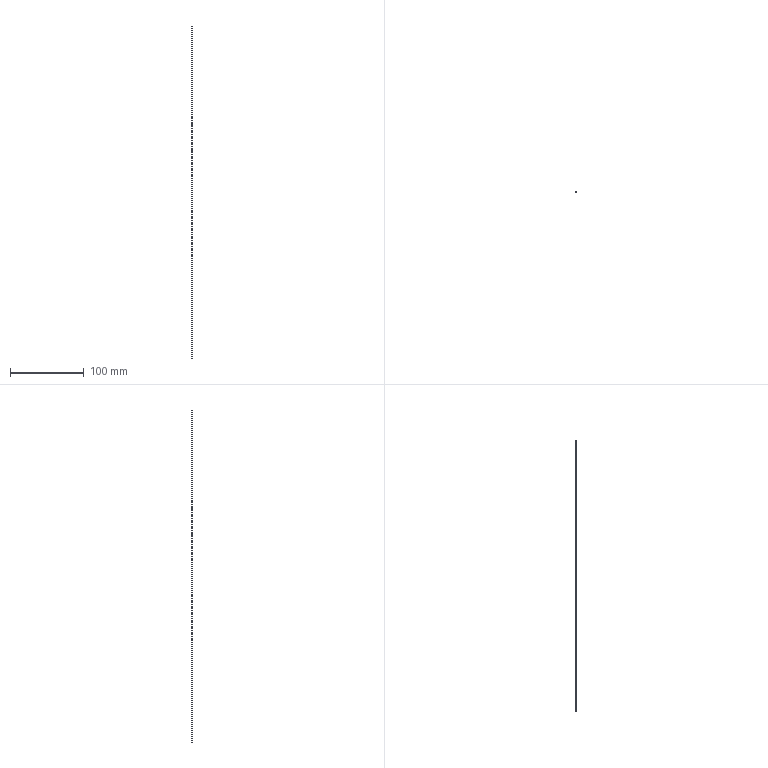Part | STEP file | LR-ZH500CP-Part-2-2 | 1 solid | 4 faces | box 1 x 1 x 450 mm | volume 353.429 mm3 | cylinder 2 | plane 2 | commonest cylinder face diameters 1 x2
STEP:
#1=CARTESIAN_POINT('',(0.,4.4,0.));
#2=VERTEX_POINT('',#1);
#3=CARTESIAN_POINT('',(0.,5.4,0.));
#4=VERTEX_POINT('',#3);
#5=CARTESIAN_POINT('',(0.,4.9,0.));
#6=DIRECTION('',(0.,0.,1.));
#7=DIRECTION('',(0.,-1.,0.));
#8=AXIS2_PLACEMENT_3D('',#5,#6,#7);
#9=CIRCLE('',#8,0.5);
#10=EDGE_CURVE('',#2,#4,#9,.T.);
#11=ORIENTED_EDGE('',*,*,#10,.T.);
#12=CARTESIAN_POINT('',(0.,5.4,450.));
#13=VERTEX_POINT('',#12);
#14=CARTESIAN_POINT('',(0.,5.4,0.));
#15=DIRECTION('',(0.,0.,1.));
#16=VECTOR('',#15,1000.);
#17=LINE('',#14,#16);
#18=EDGE_CURVE('',#4,#13,#17,.T.);
#19=ORIENTED_EDGE('',*,*,#18,.T.);
#20=CARTESIAN_POINT('',(0.,4.4,450.));
#21=VERTEX_POINT('',#20);
#22=CARTESIAN_POINT('',(0.,4.9,450.));
#23=DIRECTION('',(0.,0.,-1.));
#24=DIRECTION('',(0.,1.,0.));
#25=AXIS2_PLACEMENT_3D('',#22,#23,#24);
#26=CIRCLE('',#25,0.5);
#27=EDGE_CURVE('',#13,#21,#26,.T.);
#28=ORIENTED_EDGE('',*,*,#27,.T.);
#29=CARTESIAN_POINT('',(0.,4.4,0.));
#30=DIRECTION('',(0.,0.,1.));
#31=VECTOR('',#30,1000.);
#32=LINE('',#29,#31);
#33=EDGE_CURVE('',#2,#21,#32,.T.);
#34=ORIENTED_EDGE('',*,*,#33,.F.);
#35=EDGE_LOOP('',(#11,#19,#28,#34));
#36=FACE_OUTER_BOUND('',#35,.T.);
#37=CARTESIAN_POINT('',(0.,4.9,0.));
#38=DIRECTION('',(0.,0.,1.));
#39=DIRECTION('',(0.,-1.,0.));
#40=AXIS2_PLACEMENT_3D('',#37,#38,#39);
#41=CYLINDRICAL_SURFACE('',#40,0.5);
#42=ADVANCED_FACE('',(#36),#41,.T.);
#43=CARTESIAN_POINT('',(0.,4.9,450.));
#44=DIRECTION('',(0.,0.,-1.));
#45=DIRECTION('',(0.,1.,0.));
#46=AXIS2_PLACEMENT_3D('',#43,#44,#45);
#47=CIRCLE('',#46,0.5);
#48=EDGE_CURVE('',#21,#13,#47,.T.);
#49=ORIENTED_EDGE('',*,*,#48,.F.);
#50=ORIENTED_EDGE('',*,*,#27,.F.);
#51=EDGE_LOOP('',(#49,#50));
#52=FACE_OUTER_BOUND('',#51,.T.);
#53=CARTESIAN_POINT('',(0.,4.9,450.));
#54=DIRECTION('',(0.,0.,1.));
#55=DIRECTION('',(0.,-1.,0.));
#56=AXIS2_PLACEMENT_3D('',#53,#54,#55);
#57=PLANE('',#56);
#58=ADVANCED_FACE('',(#52),#57,.T.);
#59=ORIENTED_EDGE('',*,*,#10,.F.);
#60=CARTESIAN_POINT('',(0.,4.9,0.));
#61=DIRECTION('',(0.,0.,1.));
#62=DIRECTION('',(0.,-1.,0.));
#63=AXIS2_PLACEMENT_3D('',#60,#61,#62);
#64=CIRCLE('',#63,0.5);
#65=EDGE_CURVE('',#4,#2,#64,.T.);
#66=ORIENTED_EDGE('',*,*,#65,.F.);
#67=EDGE_LOOP('',(#59,#66));
#68=FACE_OUTER_BOUND('',#67,.T.);
#69=CARTESIAN_POINT('',(0.,4.9,0.));
#70=DIRECTION('',(0.,0.,-1.));
#71=DIRECTION('',(0.,1.,0.));
#72=AXIS2_PLACEMENT_3D('',#69,#70,#71);
#73=PLANE('',#72);
#74=ADVANCED_FACE('',(#68),#73,.T.);
#75=ORIENTED_EDGE('',*,*,#18,.F.);
#76=ORIENTED_EDGE('',*,*,#65,.T.);
#77=ORIENTED_EDGE('',*,*,#33,.T.);
#78=ORIENTED_EDGE('',*,*,#48,.T.);
#79=EDGE_LOOP('',(#75,#76,#77,#78));
#80=FACE_OUTER_BOUND('',#79,.T.);
#81=CARTESIAN_POINT('',(0.,4.9,0.));
#82=DIRECTION('',(0.,0.,1.));
#83=DIRECTION('',(0.,-1.,0.));
#84=AXIS2_PLACEMENT_3D('',#81,#82,#83);
#85=CYLINDRICAL_SURFACE('',#84,0.5);
#86=ADVANCED_FACE('',(#80),#85,.T.);
#87=CLOSED_SHELL('',(#42,#58,#74,#86));
#88=MANIFOLD_SOLID_BREP('',#87);
#89=CARTESIAN_POINT('',(0.,0.,0.));
#90=DIRECTION('',(0.,0.,1.));
#91=DIRECTION('',(1.,0.,0.));
#92=AXIS2_PLACEMENT_3D('',#89,#90,#91);
#93=(LENGTH_UNIT()NAMED_UNIT(*)SI_UNIT(.MILLI.,.METRE.));
#94=UNCERTAINTY_MEASURE_WITH_UNIT(LENGTH_MEASURE(0.00001),#93,'','');
#95=(NAMED_UNIT(*)PLANE_ANGLE_UNIT()SI_UNIT($,.RADIAN.));
#96=(NAMED_UNIT(*)SI_UNIT($,.STERADIAN.)SOLID_ANGLE_UNIT());
#97=(GEOMETRIC_REPRESENTATION_CONTEXT(3)GLOBAL_UNCERTAINTY_ASSIGNED_CONTEXT((#94))GLOBAL_UNIT_ASSIGNED_CONTEXT((#93,#95,#96))REPRESENTATION_CONTEXT('',''));
#98=ADVANCED_BREP_SHAPE_REPRESENTATION('',(#88,#92),#97);